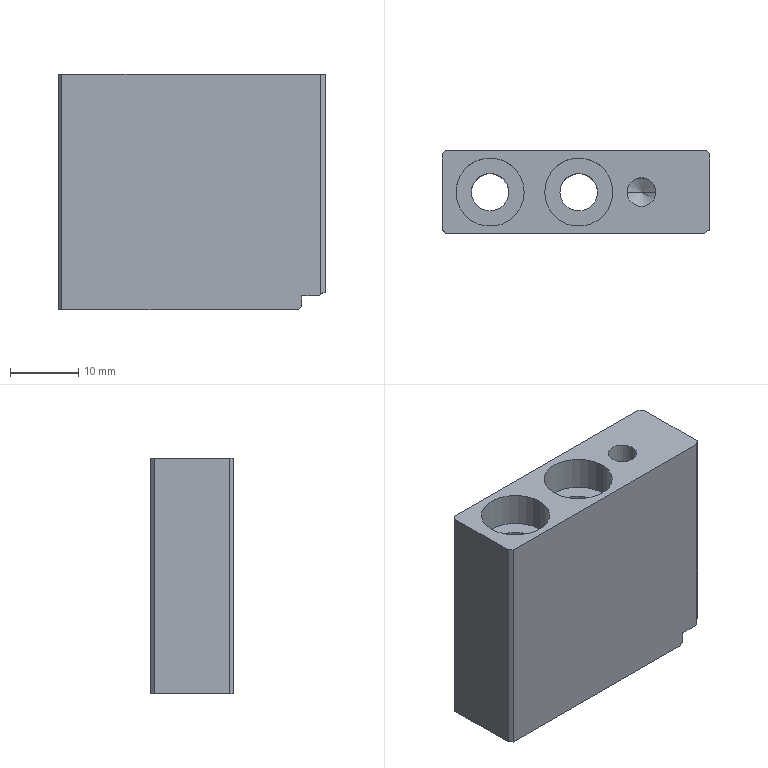Part | STEP file | side block 3-2 | 1 solid | 29 faces | box 39.2 x 12.1 x 34.5 mm | volume 13891 mm3 | plane 17 | cylinder 10 | cone 2 | commonest cylinder face diameters 5.5 x4 10 x4 4.2 x2